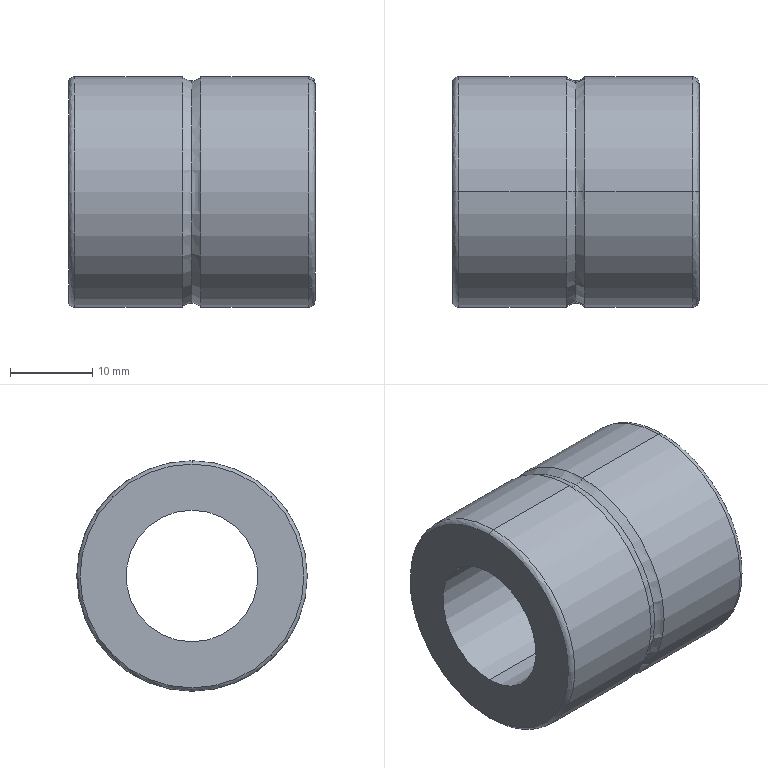Part | STEP file | LMUT16 | 1 solid | 16 faces | box 29.9 x 28 x 28 mm | volume 12313 mm3 | spline 9 | cylinder 6 | plane 1 | commonest cylinder face diameters 28 x4 16 x2